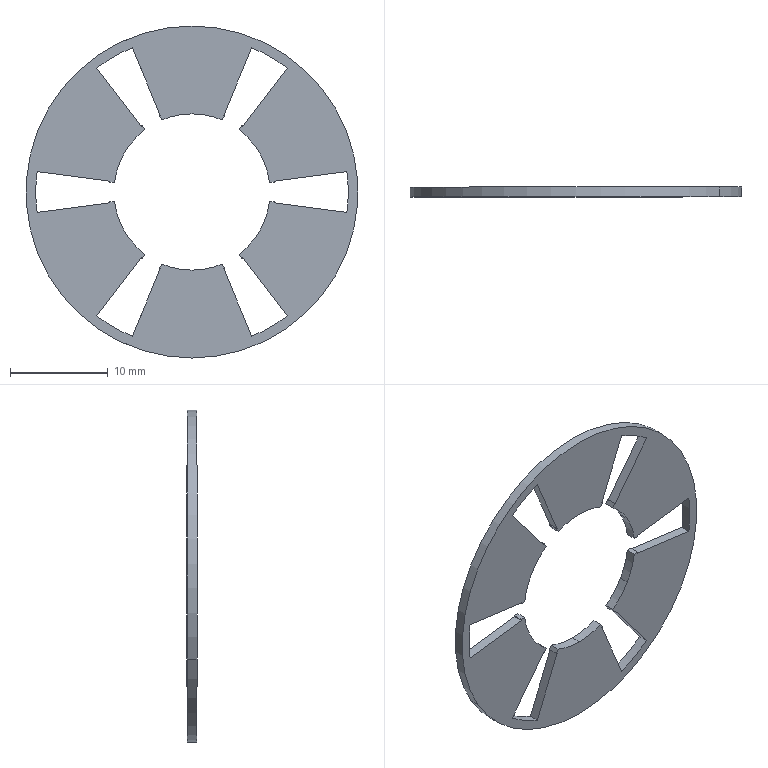Part | SolidWorks | features BaseBody 1 | 1 solid | 58 faces | box 34.001 x 1.033 x 34 mm | volume 556.527 mm3 | cylinder 32 | plane 26 | commonest cylinder face diameters 16 x12 17 x12 32 x6 34 x2